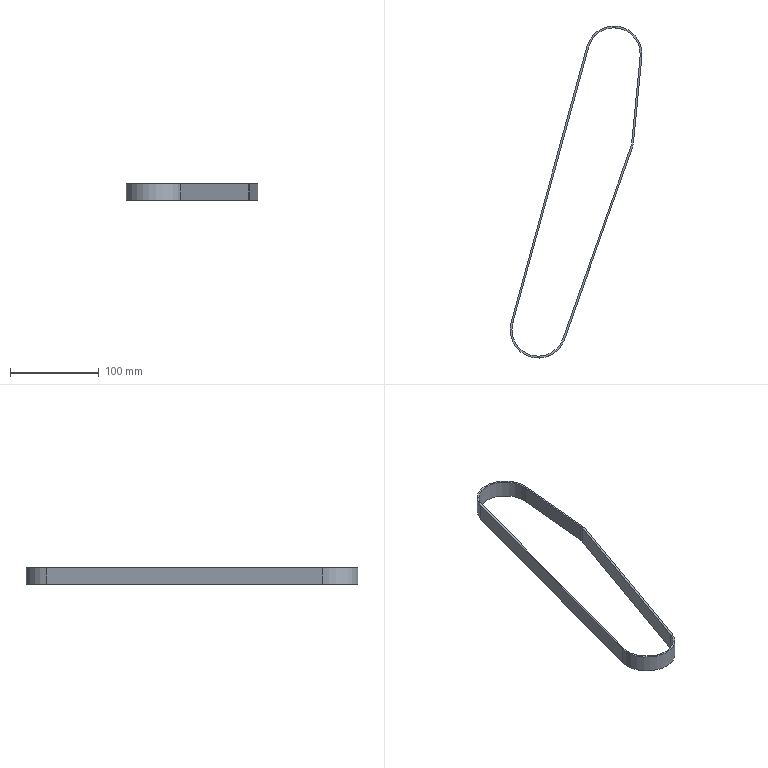Part | SolidWorks | features BaseBody 1 | 1 solid | 14 faces | box 148.838 x 374.646 x 19.05 mm | volume 32527 mm3 | plane 8 | cylinder 6 | commonest cylinder face diameters 59.266 x2 63.33 x2 39.054 x1 43.118 x1
STEP:
#1=CARTESIAN_POINT('',(115.001,308.445,9.525));
#2=VERTEX_POINT('',#1);
#3=CARTESIAN_POINT('',(115.001,308.445,-9.525));
#4=VERTEX_POINT('',#3);
#5=CARTESIAN_POINT('',(115.001,308.445,9.525));
#6=DIRECTION('',(0.,0.,-1.));
#7=VECTOR('',#6,1000.);
#8=LINE('',#5,#7);
#9=EDGE_CURVE('',#2,#4,#8,.T.);
#10=ORIENTED_EDGE('',*,*,#9,.F.);
#11=CARTESIAN_POINT('',(56.932,319.164,9.525));
#12=VERTEX_POINT('',#11);
#13=CARTESIAN_POINT('',(85.507,311.315,9.525));
#14=DIRECTION('',(0.,0.,-1.));
#15=DIRECTION('',(-0.9953,0.09688,0.));
#16=AXIS2_PLACEMENT_3D('',#13,#14,#15);
#17=CIRCLE('',#16,29.633);
#18=EDGE_CURVE('',#12,#2,#17,.T.);
#19=ORIENTED_EDGE('',*,*,#18,.F.);
#20=CARTESIAN_POINT('',(56.932,319.164,-9.525));
#21=VERTEX_POINT('',#20);
#22=CARTESIAN_POINT('',(56.932,319.164,9.525));
#23=DIRECTION('',(0.,0.,1.));
#24=VECTOR('',#23,1000.);
#25=LINE('',#22,#24);
#26=EDGE_CURVE('',#21,#12,#25,.T.);
#27=ORIENTED_EDGE('',*,*,#26,.F.);
#28=CARTESIAN_POINT('',(85.507,311.315,-9.525));
#29=DIRECTION('',(0.,0.,-1.));
#30=DIRECTION('',(-0.9953,0.09688,0.));
#31=AXIS2_PLACEMENT_3D('',#28,#29,#30);
#32=CIRCLE('',#31,29.633);
#33=EDGE_CURVE('',#21,#4,#32,.T.);
#34=ORIENTED_EDGE('',*,*,#33,.T.);
#35=EDGE_LOOP('',(#10,#19,#27,#34));
#36=FACE_OUTER_BOUND('',#35,.T.);
#37=CARTESIAN_POINT('',(85.507,311.315,0.));
#38=DIRECTION('',(0.,0.,1.));
#39=DIRECTION('',(-0.9953,0.09688,0.));
#40=AXIS2_PLACEMENT_3D('',#37,#38,#39);
#41=CYLINDRICAL_SURFACE('',#40,29.633);
#42=ADVANCED_FACE('',(#36),#41,.F.);
#43=CARTESIAN_POINT('',(117.024,308.248,-9.525));
#44=VERTEX_POINT('',#43);
#45=CARTESIAN_POINT('',(117.024,308.248,9.525));
#46=VERTEX_POINT('',#45);
#47=CARTESIAN_POINT('',(117.024,308.248,-9.525));
#48=DIRECTION('',(0.,0.,1.));
#49=VECTOR('',#48,1000.);
#50=LINE('',#47,#49);
#51=EDGE_CURVE('',#44,#46,#50,.T.);
#52=ORIENTED_EDGE('',*,*,#51,.F.);
#53=CARTESIAN_POINT('',(54.973,319.702,-9.525));
#54=VERTEX_POINT('',#53);
#55=CARTESIAN_POINT('',(85.507,311.315,-9.525));
#56=DIRECTION('',(0.,0.,-1.));
#57=DIRECTION('',(-0.9953,0.09688,0.));
#58=AXIS2_PLACEMENT_3D('',#55,#56,#57);
#59=CIRCLE('',#58,31.665);
#60=EDGE_CURVE('',#54,#44,#59,.T.);
#61=ORIENTED_EDGE('',*,*,#60,.F.);
#62=CARTESIAN_POINT('',(54.973,319.702,9.525));
#63=VERTEX_POINT('',#62);
#64=CARTESIAN_POINT('',(54.973,319.702,-9.525));
#65=DIRECTION('',(0.,0.,-1.));
#66=VECTOR('',#65,1000.);
#67=LINE('',#64,#66);
#68=EDGE_CURVE('',#63,#54,#67,.T.);
#69=ORIENTED_EDGE('',*,*,#68,.F.);
#70=CARTESIAN_POINT('',(85.507,311.315,9.525));
#71=DIRECTION('',(0.,0.,-1.));
#72=DIRECTION('',(-0.9953,0.09688,0.));
#73=AXIS2_PLACEMENT_3D('',#70,#71,#72);
#74=CIRCLE('',#73,31.665);
#75=EDGE_CURVE('',#63,#46,#74,.T.);
#76=ORIENTED_EDGE('',*,*,#75,.T.);
#77=EDGE_LOOP('',(#52,#61,#69,#76));
#78=FACE_OUTER_BOUND('',#77,.T.);
#79=CARTESIAN_POINT('',(85.507,311.315,0.));
#80=DIRECTION('',(0.,0.,1.));
#81=DIRECTION('',(-0.9953,0.09688,0.));
#82=AXIS2_PLACEMENT_3D('',#79,#80,#81);
#83=CYLINDRICAL_SURFACE('',#82,31.665);
#84=ADVANCED_FACE('',(#78),#83,.T.);
#85=ORIENTED_EDGE('',*,*,#26,.T.);
#86=CARTESIAN_POINT('',(-28.575,7.849,9.525));
#87=VERTEX_POINT('',#86);
#88=CARTESIAN_POINT('',(-28.575,7.849,9.525));
#89=DIRECTION('',(0.2649,0.9643,0.));
#90=VECTOR('',#89,1000.);
#91=LINE('',#88,#90);
#92=EDGE_CURVE('',#87,#12,#91,.T.);
#93=ORIENTED_EDGE('',*,*,#92,.F.);
#94=CARTESIAN_POINT('',(-28.575,7.849,-9.525));
#95=VERTEX_POINT('',#94);
#96=CARTESIAN_POINT('',(-28.575,7.849,9.525));
#97=DIRECTION('',(0.,0.,1.));
#98=VECTOR('',#97,1000.);
#99=LINE('',#96,#98);
#100=EDGE_CURVE('',#95,#87,#99,.T.);
#101=ORIENTED_EDGE('',*,*,#100,.F.);
#102=CARTESIAN_POINT('',(-28.575,7.849,-9.525));
#103=DIRECTION('',(0.2649,0.9643,0.));
#104=VECTOR('',#103,1000.);
#105=LINE('',#102,#104);
#106=EDGE_CURVE('',#95,#21,#105,.T.);
#107=ORIENTED_EDGE('',*,*,#106,.T.);
#108=EDGE_LOOP('',(#85,#93,#101,#107));
#109=FACE_OUTER_BOUND('',#108,.T.);
#110=CARTESIAN_POINT('',(-28.575,7.849,-9.525));
#111=DIRECTION('',(0.9643,-0.2649,0.));
#112=DIRECTION('',(0.,0.,-1.));
#113=AXIS2_PLACEMENT_3D('',#110,#111,#112);
#114=PLANE('',#113);
#115=ADVANCED_FACE('',(#109),#114,.T.);
#116=ORIENTED_EDGE('',*,*,#68,.T.);
#117=CARTESIAN_POINT('',(-30.534,8.387,-9.525));
#118=VERTEX_POINT('',#117);
#119=CARTESIAN_POINT('',(-30.534,8.387,-9.525));
#120=DIRECTION('',(0.2649,0.9643,0.));
#121=VECTOR('',#120,1000.);
#122=LINE('',#119,#121);
#123=EDGE_CURVE('',#118,#54,#122,.T.);
#124=ORIENTED_EDGE('',*,*,#123,.F.);
#125=CARTESIAN_POINT('',(-30.534,8.387,9.525));
#126=VERTEX_POINT('',#125);
#127=CARTESIAN_POINT('',(-30.534,8.387,-9.525));
#128=DIRECTION('',(0.,0.,-1.));
#129=VECTOR('',#128,1000.);
#130=LINE('',#127,#129);
#131=EDGE_CURVE('',#126,#118,#130,.T.);
#132=ORIENTED_EDGE('',*,*,#131,.F.);
#133=CARTESIAN_POINT('',(-30.534,8.387,9.525));
#134=DIRECTION('',(0.2649,0.9643,0.));
#135=VECTOR('',#134,1000.);
#136=LINE('',#133,#135);
#137=EDGE_CURVE('',#126,#63,#136,.T.);
#138=ORIENTED_EDGE('',*,*,#137,.T.);
#139=EDGE_LOOP('',(#116,#124,#132,#138));
#140=FACE_OUTER_BOUND('',#139,.T.);
#141=CARTESIAN_POINT('',(-30.534,8.387,9.525));
#142=DIRECTION('',(-0.9643,0.2649,0.));
#143=DIRECTION('',(0.,0.,1.));
#144=AXIS2_PLACEMENT_3D('',#141,#142,#143);
#145=PLANE('',#144);
#146=ADVANCED_FACE('',(#140),#145,.T.);
#147=ORIENTED_EDGE('',*,*,#100,.T.);
#148=CARTESIAN_POINT('',(27.937,-9.882,9.525));
#149=VERTEX_POINT('',#148);
#150=CARTESIAN_POINT('',(0.,0.,9.525));
#151=DIRECTION('',(0.,0.,-1.));
#152=DIRECTION('',(0.9643,-0.2649,0.));
#153=AXIS2_PLACEMENT_3D('',#150,#151,#152);
#154=CIRCLE('',#153,29.633);
#155=EDGE_CURVE('',#149,#87,#154,.T.);
#156=ORIENTED_EDGE('',*,*,#155,.F.);
#157=CARTESIAN_POINT('',(27.937,-9.882,-9.525));
#158=VERTEX_POINT('',#157);
#159=CARTESIAN_POINT('',(27.937,-9.882,9.525));
#160=DIRECTION('',(0.,0.,1.));
#161=VECTOR('',#160,1000.);
#162=LINE('',#159,#161);
#163=EDGE_CURVE('',#158,#149,#162,.T.);
#164=ORIENTED_EDGE('',*,*,#163,.F.);
#165=CARTESIAN_POINT('',(0.,0.,-9.525));
#166=DIRECTION('',(0.,0.,-1.));
#167=DIRECTION('',(0.9643,-0.2649,0.));
#168=AXIS2_PLACEMENT_3D('',#165,#166,#167);
#169=CIRCLE('',#168,29.633);
#170=EDGE_CURVE('',#158,#95,#169,.T.);
#171=ORIENTED_EDGE('',*,*,#170,.T.);
#172=EDGE_LOOP('',(#147,#156,#164,#171));
#173=FACE_OUTER_BOUND('',#172,.T.);
#174=CARTESIAN_POINT('',(0.,0.,0.));
#175=DIRECTION('',(0.,0.,1.));
#176=DIRECTION('',(0.9643,-0.2649,0.));
#177=AXIS2_PLACEMENT_3D('',#174,#175,#176);
#178=CYLINDRICAL_SURFACE('',#177,29.633);
#179=ADVANCED_FACE('',(#173),#178,.F.);
#180=ORIENTED_EDGE('',*,*,#131,.T.);
#181=CARTESIAN_POINT('',(29.853,-10.56,-9.525));
#182=VERTEX_POINT('',#181);
#183=CARTESIAN_POINT('',(0.,0.,-9.525));
#184=DIRECTION('',(0.,0.,-1.));
#185=DIRECTION('',(0.9643,-0.2649,0.));
#186=AXIS2_PLACEMENT_3D('',#183,#184,#185);
#187=CIRCLE('',#186,31.665);
#188=EDGE_CURVE('',#182,#118,#187,.T.);
#189=ORIENTED_EDGE('',*,*,#188,.F.);
#190=CARTESIAN_POINT('',(29.853,-10.56,9.525));
#191=VERTEX_POINT('',#190);
#192=CARTESIAN_POINT('',(29.853,-10.56,-9.525));
#193=DIRECTION('',(0.,0.,-1.));
#194=VECTOR('',#193,1000.);
#195=LINE('',#192,#194);
#196=EDGE_CURVE('',#191,#182,#195,.T.);
#197=ORIENTED_EDGE('',*,*,#196,.F.);
#198=CARTESIAN_POINT('',(0.,0.,9.525));
#199=DIRECTION('',(0.,0.,-1.));
#200=DIRECTION('',(0.9643,-0.2649,0.));
#201=AXIS2_PLACEMENT_3D('',#198,#199,#200);
#202=CIRCLE('',#201,31.665);
#203=EDGE_CURVE('',#191,#126,#202,.T.);
#204=ORIENTED_EDGE('',*,*,#203,.T.);
#205=EDGE_LOOP('',(#180,#189,#197,#204));
#206=FACE_OUTER_BOUND('',#205,.T.);
#207=CARTESIAN_POINT('',(0.,0.,0.));
#208=DIRECTION('',(0.,0.,1.));
#209=DIRECTION('',(0.9643,-0.2649,0.));
#210=AXIS2_PLACEMENT_3D('',#207,#208,#209);
#211=CYLINDRICAL_SURFACE('',#210,31.665);
#212=ADVANCED_FACE('',(#206),#211,.T.);
#213=ORIENTED_EDGE('',*,*,#163,.T.);
#214=CARTESIAN_POINT('',(104.51,206.587,9.525));
#215=VERTEX_POINT('',#214);
#216=CARTESIAN_POINT('',(104.51,206.587,9.525));
#217=DIRECTION('',(-0.3335,-0.9428,0.));
#218=VECTOR('',#217,1000.);
#219=LINE('',#216,#218);
#220=EDGE_CURVE('',#215,#149,#219,.T.);
#221=ORIENTED_EDGE('',*,*,#220,.F.);
#222=CARTESIAN_POINT('',(104.51,206.587,-9.525));
#223=VERTEX_POINT('',#222);
#224=CARTESIAN_POINT('',(104.51,206.587,9.525));
#225=DIRECTION('',(0.,0.,1.));
#226=VECTOR('',#225,1000.);
#227=LINE('',#224,#226);
#228=EDGE_CURVE('',#223,#215,#227,.T.);
#229=ORIENTED_EDGE('',*,*,#228,.F.);
#230=CARTESIAN_POINT('',(104.51,206.587,-9.525));
#231=DIRECTION('',(-0.3335,-0.9428,0.));
#232=VECTOR('',#231,1000.);
#233=LINE('',#230,#232);
#234=EDGE_CURVE('',#223,#158,#233,.T.);
#235=ORIENTED_EDGE('',*,*,#234,.T.);
#236=EDGE_LOOP('',(#213,#221,#229,#235));
#237=FACE_OUTER_BOUND('',#236,.T.);
#238=CARTESIAN_POINT('',(104.51,206.587,-9.525));
#239=DIRECTION('',(-0.9428,0.3335,0.));
#240=DIRECTION('',(0.,0.,1.));
#241=AXIS2_PLACEMENT_3D('',#238,#239,#240);
#242=PLANE('',#241);
#243=ADVANCED_FACE('',(#237),#242,.T.);
#244=ORIENTED_EDGE('',*,*,#196,.T.);
#245=CARTESIAN_POINT('',(106.426,205.909,-9.525));
#246=VERTEX_POINT('',#245);
#247=CARTESIAN_POINT('',(106.426,205.909,-9.525));
#248=DIRECTION('',(-0.3335,-0.9428,0.));
#249=VECTOR('',#248,1000.);
#250=LINE('',#247,#249);
#251=EDGE_CURVE('',#246,#182,#250,.T.);
#252=ORIENTED_EDGE('',*,*,#251,.F.);
#253=CARTESIAN_POINT('',(106.426,205.909,9.525));
#254=VERTEX_POINT('',#253);
#255=CARTESIAN_POINT('',(106.426,205.909,-9.525));
#256=DIRECTION('',(0.,0.,-1.));
#257=VECTOR('',#256,1000.);
#258=LINE('',#255,#257);
#259=EDGE_CURVE('',#254,#246,#258,.T.);
#260=ORIENTED_EDGE('',*,*,#259,.F.);
#261=CARTESIAN_POINT('',(106.426,205.909,9.525));
#262=DIRECTION('',(-0.3335,-0.9428,0.));
#263=VECTOR('',#262,1000.);
#264=LINE('',#261,#263);
#265=EDGE_CURVE('',#254,#191,#264,.T.);
#266=ORIENTED_EDGE('',*,*,#265,.T.);
#267=EDGE_LOOP('',(#244,#252,#260,#266));
#268=FACE_OUTER_BOUND('',#267,.T.);
#269=CARTESIAN_POINT('',(106.426,205.909,9.525));
#270=DIRECTION('',(0.9428,-0.3335,0.));
#271=DIRECTION('',(0.,0.,-1.));
#272=AXIS2_PLACEMENT_3D('',#269,#270,#271);
#273=PLANE('',#272);
#274=ADVANCED_FACE('',(#268),#273,.T.);
#275=CARTESIAN_POINT('',(105.536,211.207,-9.525));
#276=VERTEX_POINT('',#275);
#277=CARTESIAN_POINT('',(115.001,308.445,-9.525));
#278=DIRECTION('',(-0.09688,-0.9953,0.));
#279=VECTOR('',#278,1000.);
#280=LINE('',#277,#279);
#281=EDGE_CURVE('',#4,#276,#280,.T.);
#282=ORIENTED_EDGE('',*,*,#281,.F.);
#283=ORIENTED_EDGE('',*,*,#33,.F.);
#284=ORIENTED_EDGE('',*,*,#106,.F.);
#285=ORIENTED_EDGE('',*,*,#170,.F.);
#286=ORIENTED_EDGE('',*,*,#234,.F.);
#287=CARTESIAN_POINT('',(86.101,213.099,-9.525));
#288=DIRECTION('',(0.,0.,-1.));
#289=DIRECTION('',(-0.9428,0.3335,0.));
#290=AXIS2_PLACEMENT_3D('',#287,#288,#289);
#291=CIRCLE('',#290,19.527);
#292=EDGE_CURVE('',#276,#223,#291,.T.);
#293=ORIENTED_EDGE('',*,*,#292,.F.);
#294=EDGE_LOOP('',(#282,#283,#284,#285,#286,#293));
#295=FACE_BOUND('',#294,.T.);
#296=CARTESIAN_POINT('',(107.559,211.01,-9.525));
#297=VERTEX_POINT('',#296);
#298=CARTESIAN_POINT('',(86.101,213.099,-9.525));
#299=DIRECTION('',(0.,0.,-1.));
#300=DIRECTION('',(-0.9428,0.3335,0.));
#301=AXIS2_PLACEMENT_3D('',#298,#299,#300);
#302=CIRCLE('',#301,21.559);
#303=EDGE_CURVE('',#297,#246,#302,.T.);
#304=ORIENTED_EDGE('',*,*,#303,.T.);
#305=ORIENTED_EDGE('',*,*,#251,.T.);
#306=ORIENTED_EDGE('',*,*,#188,.T.);
#307=ORIENTED_EDGE('',*,*,#123,.T.);
#308=ORIENTED_EDGE('',*,*,#60,.T.);
#309=CARTESIAN_POINT('',(117.024,308.248,-9.525));
#310=DIRECTION('',(-0.09688,-0.9953,0.));
#311=VECTOR('',#310,1000.);
#312=LINE('',#309,#311);
#313=EDGE_CURVE('',#44,#297,#312,.T.);
#314=ORIENTED_EDGE('',*,*,#313,.T.);
#315=EDGE_LOOP('',(#304,#305,#306,#307,#308,#314));
#316=FACE_OUTER_BOUND('',#315,.T.);
#317=CARTESIAN_POINT('',(106.548,211.109,-9.525));
#318=DIRECTION('',(0.,0.,-1.));
#319=DIRECTION('',(0.,-1.,0.));
#320=AXIS2_PLACEMENT_3D('',#317,#318,#319);
#321=PLANE('',#320);
#322=ADVANCED_FACE('',(#295,#316),#321,.T.);
#323=ORIENTED_EDGE('',*,*,#228,.T.);
#324=CARTESIAN_POINT('',(105.536,211.207,9.525));
#325=VERTEX_POINT('',#324);
#326=CARTESIAN_POINT('',(86.101,213.099,9.525));
#327=DIRECTION('',(0.,0.,-1.));
#328=DIRECTION('',(-0.9428,0.3335,0.));
#329=AXIS2_PLACEMENT_3D('',#326,#327,#328);
#330=CIRCLE('',#329,19.527);
#331=EDGE_CURVE('',#325,#215,#330,.T.);
#332=ORIENTED_EDGE('',*,*,#331,.F.);
#333=CARTESIAN_POINT('',(105.536,211.207,9.525));
#334=DIRECTION('',(0.,0.,1.));
#335=VECTOR('',#334,1000.);
#336=LINE('',#333,#335);
#337=EDGE_CURVE('',#276,#325,#336,.T.);
#338=ORIENTED_EDGE('',*,*,#337,.F.);
#339=ORIENTED_EDGE('',*,*,#292,.T.);
#340=EDGE_LOOP('',(#323,#332,#338,#339));
#341=FACE_OUTER_BOUND('',#340,.T.);
#342=CARTESIAN_POINT('',(86.101,213.099,0.));
#343=DIRECTION('',(0.,0.,1.));
#344=DIRECTION('',(-0.9428,0.3335,0.));
#345=AXIS2_PLACEMENT_3D('',#342,#343,#344);
#346=CYLINDRICAL_SURFACE('',#345,19.527);
#347=ADVANCED_FACE('',(#341),#346,.F.);
#348=ORIENTED_EDGE('',*,*,#331,.T.);
#349=ORIENTED_EDGE('',*,*,#220,.T.);
#350=ORIENTED_EDGE('',*,*,#155,.T.);
#351=ORIENTED_EDGE('',*,*,#92,.T.);
#352=ORIENTED_EDGE('',*,*,#18,.T.);
#353=CARTESIAN_POINT('',(115.001,308.445,9.525));
#354=DIRECTION('',(-0.09688,-0.9953,0.));
#355=VECTOR('',#354,1000.);
#356=LINE('',#353,#355);
#357=EDGE_CURVE('',#2,#325,#356,.T.);
#358=ORIENTED_EDGE('',*,*,#357,.T.);
#359=EDGE_LOOP('',(#348,#349,#350,#351,#352,#358));
#360=FACE_BOUND('',#359,.T.);
#361=CARTESIAN_POINT('',(107.559,211.01,9.525));
#362=VERTEX_POINT('',#361);
#363=CARTESIAN_POINT('',(117.024,308.248,9.525));
#364=DIRECTION('',(-0.09688,-0.9953,0.));
#365=VECTOR('',#364,1000.);
#366=LINE('',#363,#365);
#367=EDGE_CURVE('',#46,#362,#366,.T.);
#368=ORIENTED_EDGE('',*,*,#367,.F.);
#369=ORIENTED_EDGE('',*,*,#75,.F.);
#370=ORIENTED_EDGE('',*,*,#137,.F.);
#371=ORIENTED_EDGE('',*,*,#203,.F.);
#372=ORIENTED_EDGE('',*,*,#265,.F.);
#373=CARTESIAN_POINT('',(86.101,213.099,9.525));
#374=DIRECTION('',(0.,0.,-1.));
#375=DIRECTION('',(-0.9428,0.3335,0.));
#376=AXIS2_PLACEMENT_3D('',#373,#374,#375);
#377=CIRCLE('',#376,21.559);
#378=EDGE_CURVE('',#362,#254,#377,.T.);
#379=ORIENTED_EDGE('',*,*,#378,.F.);
#380=EDGE_LOOP('',(#368,#369,#370,#371,#372,#379));
#381=FACE_OUTER_BOUND('',#380,.T.);
#382=CARTESIAN_POINT('',(106.548,211.109,9.525));
#383=DIRECTION('',(0.,0.,1.));
#384=DIRECTION('',(1.,0.,0.));
#385=AXIS2_PLACEMENT_3D('',#382,#383,#384);
#386=PLANE('',#385);
#387=ADVANCED_FACE('',(#360,#381),#386,.T.);
#388=ORIENTED_EDGE('',*,*,#259,.T.);
#389=ORIENTED_EDGE('',*,*,#303,.F.);
#390=CARTESIAN_POINT('',(107.559,211.01,-9.525));
#391=DIRECTION('',(0.,0.,-1.));
#392=VECTOR('',#391,1000.);
#393=LINE('',#390,#392);
#394=EDGE_CURVE('',#362,#297,#393,.T.);
#395=ORIENTED_EDGE('',*,*,#394,.F.);
#396=ORIENTED_EDGE('',*,*,#378,.T.);
#397=EDGE_LOOP('',(#388,#389,#395,#396));
#398=FACE_OUTER_BOUND('',#397,.T.);
#399=CARTESIAN_POINT('',(86.101,213.099,0.));
#400=DIRECTION('',(0.,0.,1.));
#401=DIRECTION('',(-0.9428,0.3335,0.));
#402=AXIS2_PLACEMENT_3D('',#399,#400,#401);
#403=CYLINDRICAL_SURFACE('',#402,21.559);
#404=ADVANCED_FACE('',(#398),#403,.T.);
#405=ORIENTED_EDGE('',*,*,#337,.T.);
#406=ORIENTED_EDGE('',*,*,#357,.F.);
#407=ORIENTED_EDGE('',*,*,#9,.T.);
#408=ORIENTED_EDGE('',*,*,#281,.T.);
#409=EDGE_LOOP('',(#405,#406,#407,#408));
#410=FACE_OUTER_BOUND('',#409,.T.);
#411=CARTESIAN_POINT('',(115.001,308.445,-9.525));
#412=DIRECTION('',(-0.9953,0.09688,0.));
#413=DIRECTION('',(0.,0.,1.));
#414=AXIS2_PLACEMENT_3D('',#411,#412,#413);
#415=PLANE('',#414);
#416=ADVANCED_FACE('',(#410),#415,.T.);
#417=ORIENTED_EDGE('',*,*,#394,.T.);
#418=ORIENTED_EDGE('',*,*,#313,.F.);
#419=ORIENTED_EDGE('',*,*,#51,.T.);
#420=ORIENTED_EDGE('',*,*,#367,.T.);
#421=EDGE_LOOP('',(#417,#418,#419,#420));
#422=FACE_OUTER_BOUND('',#421,.T.);
#423=CARTESIAN_POINT('',(117.024,308.248,9.525));
#424=DIRECTION('',(0.9953,-0.09688,0.));
#425=DIRECTION('',(0.,0.,-1.));
#426=AXIS2_PLACEMENT_3D('',#423,#424,#425);
#427=PLANE('',#426);
#428=ADVANCED_FACE('',(#422),#427,.T.);
#429=CLOSED_SHELL('',(#42,#84,#115,#146,#179,#212,#243,#274,#322,#347,#387,#404,#416,#428));
#430=MANIFOLD_SOLID_BREP('',#429);
#431=CARTESIAN_POINT('',(0.,0.,0.));
#432=DIRECTION('',(0.,0.,1.));
#433=DIRECTION('',(1.,0.,0.));
#434=AXIS2_PLACEMENT_3D('',#431,#432,#433);
#435=(LENGTH_UNIT()NAMED_UNIT(*)SI_UNIT(.MILLI.,.METRE.));
#436=UNCERTAINTY_MEASURE_WITH_UNIT(LENGTH_MEASURE(0.00001),#435,'','');
#437=(NAMED_UNIT(*)PLANE_ANGLE_UNIT()SI_UNIT($,.RADIAN.));
#438=(NAMED_UNIT(*)SI_UNIT($,.STERADIAN.)SOLID_ANGLE_UNIT());
#439=(GEOMETRIC_REPRESENTATION_CONTEXT(3)GLOBAL_UNCERTAINTY_ASSIGNED_CONTEXT((#436))GLOBAL_UNIT_ASSIGNED_CONTEXT((#435,#437,#438))REPRESENTATION_CONTEXT('',''));
#440=ADVANCED_BREP_SHAPE_REPRESENTATION('',(#430,#434),#439);